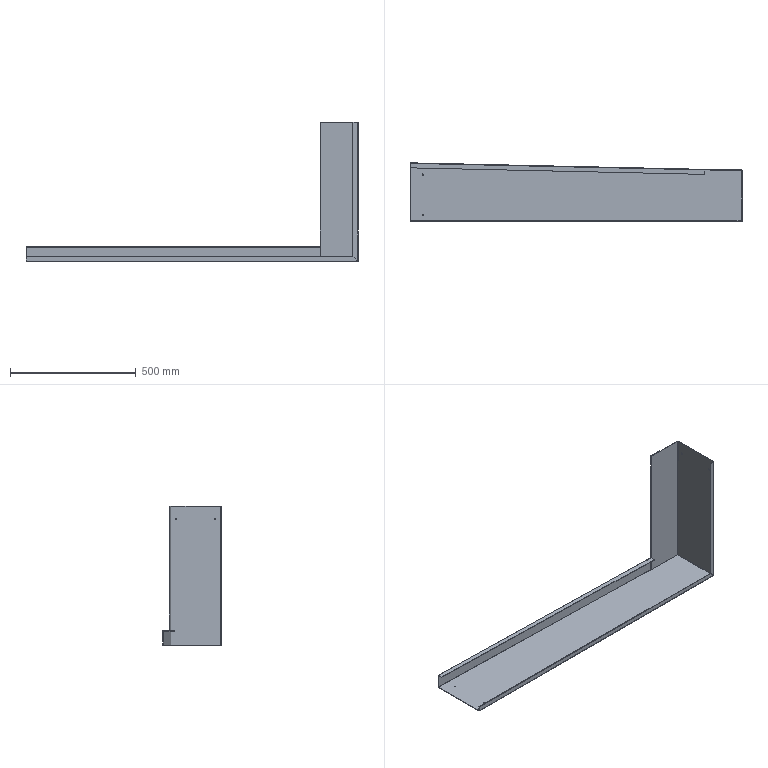Part | STEP file | TS-S51 | 1 solid | 68 faces | box 1320 x 231.983 x 555 mm | volume 1200931 mm3 | plane 45 | cylinder 20 | spline 3 | commonest cylinder face diameters 5.4 x8 0.4 x6 4.4 x6